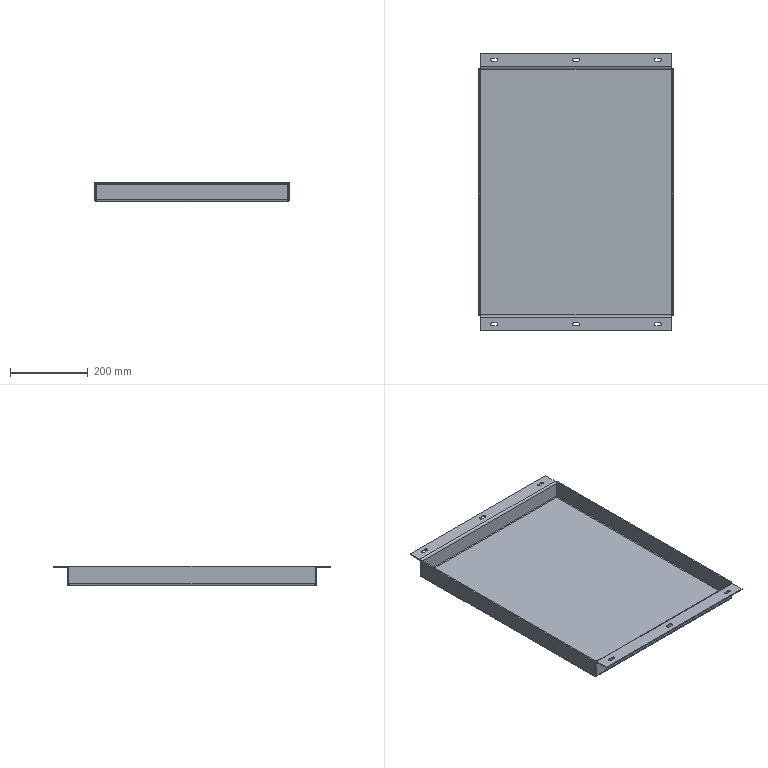Part | SolidWorks | features EdgeFlange 2, FlatPattern 1, ICE 1, SMBaseFlange 1, SheetMetal 1 | 1 solid | 84 faces | box 500 x 714 x 50 mm | volume 1369290 mm3 | plane 46 | cylinder 30 | spline 8 | commonest cylinder face diameters 8.5 x18 4 x6 10 x6